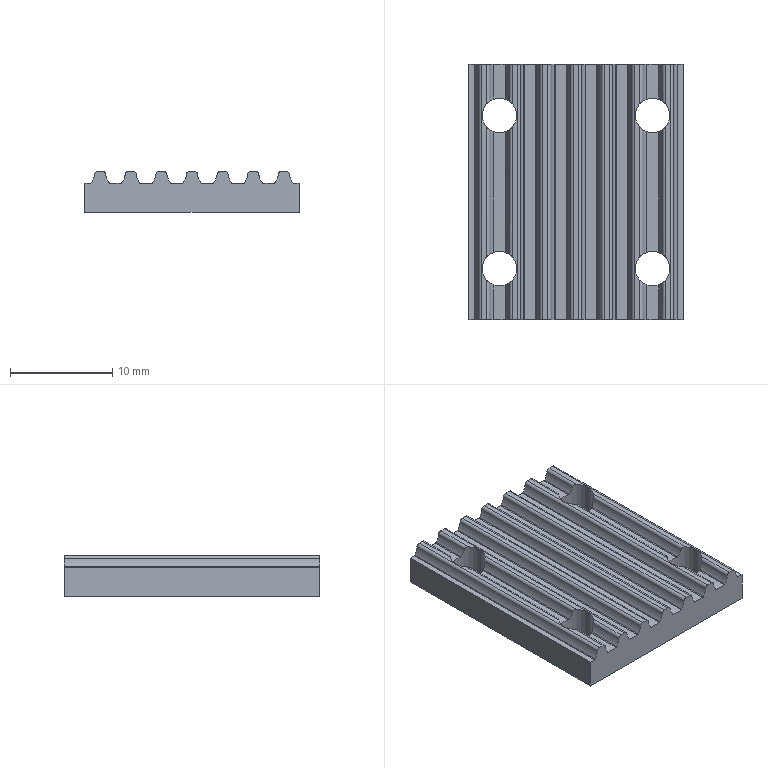Part | STEP file | C-TBCR-S3M100.stp | 1 solid | 98 faces | box 21 x 25 x 4 mm | volume 1633 mm3 | cylinder 74 | plane 24 | commonest cylinder face diameters 0.2 x22 0.6 x22 3.9 x22 3.4 x8